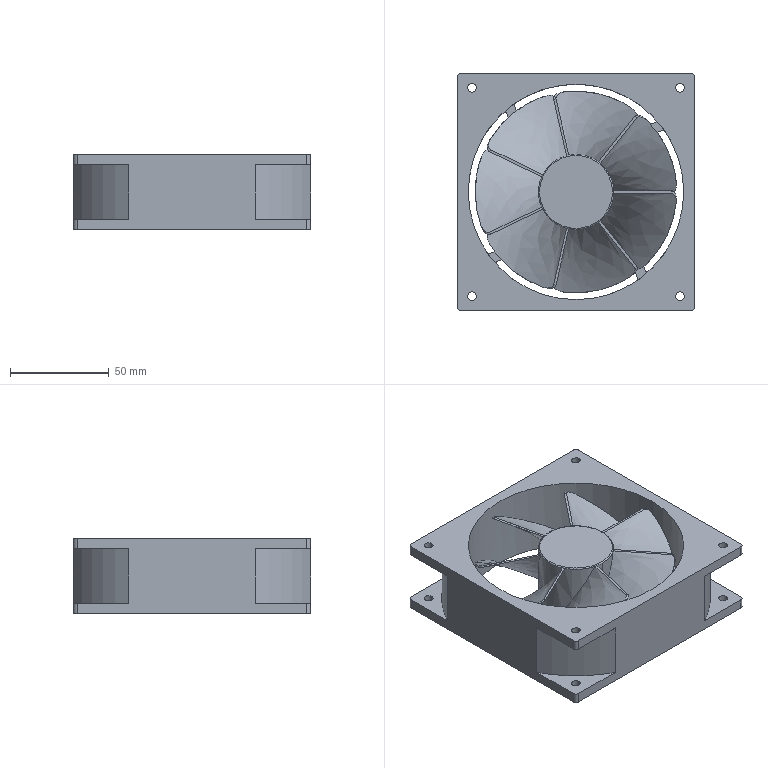Part | SolidWorks | features ICE 6, Fillet 5, CirPattern 2, RefAxis 2, BossThin 1, Extrusion 1, Helix 1, RevCut 1, Revolution 1, Sweep 1 | 1 solid | 222 faces | box 120 x 120 x 38 mm | volume 208325 mm3 | plane 107 | cylinder 59 | spline 54 | torus 2 | commonest cylinder face diameters 4.4 x16 4 x13 2 x10 38 x6 42 x4 136 x4